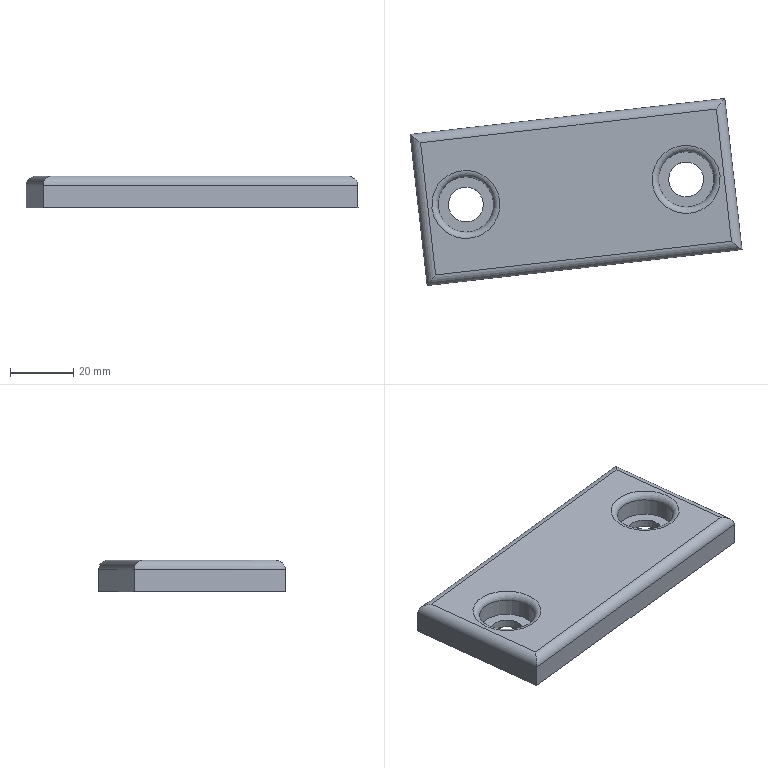Part | NX | features XQ 2 | 1 solid | 18 faces | box 104.791 x 59.012 x 10 mm | volume 43256 mm3 | plane 8 | cylinder 8 | torus 2 | commonest cylinder face diameters 6 x4 11 x2 17.5 x2
STEP:
#1=CARTESIAN_POINT('',(2747.315,315.593,-122.5));
#2=VERTEX_POINT('',#1);
#3=CARTESIAN_POINT('',(2747.315,315.593,-115.5));
#4=VERTEX_POINT('',#3);
#5=CARTESIAN_POINT('',(2747.315,315.593,-117.5));
#6=DIRECTION('',(-0.000000001,0.,1.));
#7=VECTOR('',#6,1000.);
#8=LINE('',#5,#7);
#9=EDGE_CURVE('',#2,#4,#8,.T.);
#10=ORIENTED_EDGE('',*,*,#9,.F.);
#11=CARTESIAN_POINT('',(2647.958,304.273,-122.5));
#12=VERTEX_POINT('',#11);
#13=CARTESIAN_POINT('',(2647.958,304.273,-122.5));
#14=DIRECTION('',(0.9936,0.1132,0.000000001));
#15=VECTOR('',#14,1000.);
#16=LINE('',#13,#15);
#17=EDGE_CURVE('',#12,#2,#16,.T.);
#18=ORIENTED_EDGE('',*,*,#17,.F.);
#19=CARTESIAN_POINT('',(2647.958,304.273,-115.5));
#20=VERTEX_POINT('',#19);
#21=CARTESIAN_POINT('',(2647.958,304.273,-117.5));
#22=DIRECTION('',(0.000000001,0.,-1.));
#23=VECTOR('',#22,1000.);
#24=LINE('',#21,#23);
#25=EDGE_CURVE('',#20,#12,#24,.T.);
#26=ORIENTED_EDGE('',*,*,#25,.F.);
#27=CARTESIAN_POINT('',(2647.958,304.273,-115.5));
#28=DIRECTION('',(-0.9936,-0.1132,-0.000000001));
#29=VECTOR('',#28,1000.);
#30=LINE('',#27,#29);
#31=EDGE_CURVE('',#4,#20,#30,.T.);
#32=ORIENTED_EDGE('',*,*,#31,.F.);
#33=EDGE_LOOP('',(#10,#18,#26,#32));
#34=FACE_BOUND('',#33,.T.);
#35=CARTESIAN_POINT('',(2647.958,304.273,-117.5));
#36=DIRECTION('',(-0.1132,0.9936,0.));
#37=DIRECTION('',(0.9936,0.1132,0.000000001));
#38=AXIS2_PLACEMENT_3D('',#35,#36,#37);
#39=PLANE('',#38);
#40=ADVANCED_FACE('',(#34),#39,.T.);
#41=CARTESIAN_POINT('',(2752.749,267.902,-115.5));
#42=VERTEX_POINT('',#41);
#43=CARTESIAN_POINT('',(2752.749,267.902,-122.5));
#44=VERTEX_POINT('',#43);
#45=CARTESIAN_POINT('',(2752.749,267.902,-117.5));
#46=DIRECTION('',(0.000000001,0.,-1.));
#47=VECTOR('',#46,1000.);
#48=LINE('',#45,#47);
#49=EDGE_CURVE('',#42,#44,#48,.T.);
#50=ORIENTED_EDGE('',*,*,#49,.T.);
#51=CARTESIAN_POINT('',(2750.032,291.748,-122.5));
#52=DIRECTION('',(0.1132,-0.9936,0.));
#53=VECTOR('',#52,1000.);
#54=LINE('',#51,#53);
#55=EDGE_CURVE('',#2,#44,#54,.T.);
#56=ORIENTED_EDGE('',*,*,#55,.F.);
#57=ORIENTED_EDGE('',*,*,#9,.T.);
#58=CARTESIAN_POINT('',(2750.032,291.748,-115.5));
#59=DIRECTION('',(-0.1132,0.9936,0.));
#60=VECTOR('',#59,1000.);
#61=LINE('',#58,#60);
#62=EDGE_CURVE('',#42,#4,#61,.T.);
#63=ORIENTED_EDGE('',*,*,#62,.F.);
#64=EDGE_LOOP('',(#50,#56,#57,#63));
#65=FACE_BOUND('',#64,.T.);
#66=CARTESIAN_POINT('',(2750.032,291.748,-117.5));
#67=DIRECTION('',(0.9936,0.1132,0.000000001));
#68=DIRECTION('',(0.1132,-0.9936,0.));
#69=AXIS2_PLACEMENT_3D('',#66,#67,#68);
#70=PLANE('',#69);
#71=ADVANCED_FACE('',(#65),#70,.T.);
#72=CARTESIAN_POINT('',(2724.448,288.833,-112.5));
#73=VERTEX_POINT('',#72);
#74=CARTESIAN_POINT('',(2735.129,290.05,-112.5));
#75=DIRECTION('',(-0.000000001,0.,1.));
#76=DIRECTION('',(-0.9936,-0.1132,-0.000000001));
#77=AXIS2_PLACEMENT_3D('',#74,#75,#76);
#78=CIRCLE('',#77,10.75);
#79=EDGE_CURVE('',#73,#73,#78,.T.);
#80=ORIENTED_EDGE('',*,*,#79,.F.);
#81=EDGE_LOOP('',(#80));
#82=FACE_BOUND('',#81,.T.);
#83=CARTESIAN_POINT('',(2654.898,280.908,-112.5));
#84=VERTEX_POINT('',#83);
#85=CARTESIAN_POINT('',(2665.579,282.125,-112.5));
#86=DIRECTION('',(-0.000000001,0.,1.));
#87=DIRECTION('',(-0.9936,-0.1132,-0.000000001));
#88=AXIS2_PLACEMENT_3D('',#85,#86,#87);
#89=CIRCLE('',#88,10.75);
#90=EDGE_CURVE('',#84,#84,#89,.T.);
#91=ORIENTED_EDGE('',*,*,#90,.F.);
#92=EDGE_LOOP('',(#91));
#93=FACE_BOUND('',#92,.T.);
#94=CARTESIAN_POINT('',(2749.429,270.543,-112.5));
#95=VERTEX_POINT('',#94);
#96=CARTESIAN_POINT('',(2656.033,259.902,-112.5));
#97=VERTEX_POINT('',#96);
#98=CARTESIAN_POINT('',(2653.052,259.562,-112.5));
#99=DIRECTION('',(-0.9936,-0.1132,-0.000000001));
#100=VECTOR('',#99,1000.);
#101=LINE('',#98,#100);
#102=EDGE_CURVE('',#95,#97,#101,.T.);
#103=ORIENTED_EDGE('',*,*,#102,.F.);
#104=CARTESIAN_POINT('',(2744.674,312.273,-112.5));
#105=VERTEX_POINT('',#104);
#106=CARTESIAN_POINT('',(2747.052,291.408,-112.5));
#107=DIRECTION('',(0.1132,-0.9936,0.));
#108=VECTOR('',#107,1000.);
#109=LINE('',#106,#108);
#110=EDGE_CURVE('',#105,#95,#109,.T.);
#111=ORIENTED_EDGE('',*,*,#110,.F.);
#112=CARTESIAN_POINT('',(2651.279,301.632,-112.5));
#113=VERTEX_POINT('',#112);
#114=CARTESIAN_POINT('',(2648.298,301.292,-112.5));
#115=DIRECTION('',(0.9936,0.1132,0.000000001));
#116=VECTOR('',#115,1000.);
#117=LINE('',#114,#116);
#118=EDGE_CURVE('',#113,#105,#117,.T.);
#119=ORIENTED_EDGE('',*,*,#118,.F.);
#120=CARTESIAN_POINT('',(2653.656,280.767,-112.5));
#121=DIRECTION('',(-0.1132,0.9936,0.));
#122=VECTOR('',#121,1000.);
#123=LINE('',#120,#122);
#124=EDGE_CURVE('',#97,#113,#123,.T.);
#125=ORIENTED_EDGE('',*,*,#124,.F.);
#126=EDGE_LOOP('',(#103,#111,#119,#125));
#127=FACE_BOUND('',#126,.T.);
#128=CARTESIAN_POINT('',(2650.675,280.427,-112.5));
#129=DIRECTION('',(-0.000000001,0.,1.));
#130=DIRECTION('',(0.9936,0.1132,0.000000001));
#131=AXIS2_PLACEMENT_3D('',#128,#129,#130);
#132=PLANE('',#131);
#133=ADVANCED_FACE('',(#82,#93,#127),#132,.T.);
#134=CARTESIAN_POINT('',(2653.392,256.582,-122.5));
#135=VERTEX_POINT('',#134);
#136=CARTESIAN_POINT('',(2653.392,256.582,-115.5));
#137=VERTEX_POINT('',#136);
#138=CARTESIAN_POINT('',(2653.392,256.582,-117.5));
#139=DIRECTION('',(-0.000000001,0.,1.));
#140=VECTOR('',#139,1000.);
#141=LINE('',#138,#140);
#142=EDGE_CURVE('',#135,#137,#141,.T.);
#143=ORIENTED_EDGE('',*,*,#142,.F.);
#144=CARTESIAN_POINT('',(2653.392,256.582,-122.5));
#145=DIRECTION('',(0.9936,0.1132,0.000000001));
#146=VECTOR('',#145,1000.);
#147=LINE('',#144,#146);
#148=EDGE_CURVE('',#135,#44,#147,.T.);
#149=ORIENTED_EDGE('',*,*,#148,.T.);
#150=ORIENTED_EDGE('',*,*,#49,.F.);
#151=CARTESIAN_POINT('',(2653.392,256.582,-115.5));
#152=DIRECTION('',(0.9936,0.1132,0.000000001));
#153=VECTOR('',#152,1000.);
#154=LINE('',#151,#153);
#155=EDGE_CURVE('',#137,#42,#154,.T.);
#156=ORIENTED_EDGE('',*,*,#155,.F.);
#157=EDGE_LOOP('',(#143,#149,#150,#156));
#158=FACE_BOUND('',#157,.T.);
#159=CARTESIAN_POINT('',(2653.392,256.582,-117.5));
#160=DIRECTION('',(0.1132,-0.9936,0.));
#161=DIRECTION('',(-0.9936,-0.1132,-0.000000001));
#162=AXIS2_PLACEMENT_3D('',#159,#160,#161);
#163=PLANE('',#162);
#164=ADVANCED_FACE('',(#158),#163,.T.);
#165=CARTESIAN_POINT('',(2729.664,289.427,-122.5));
#166=VERTEX_POINT('',#165);
#167=CARTESIAN_POINT('',(2735.129,290.05,-122.5));
#168=DIRECTION('',(0.000000001,0.,-1.));
#169=DIRECTION('',(-0.9936,-0.1132,-0.000000001));
#170=AXIS2_PLACEMENT_3D('',#167,#168,#169);
#171=CIRCLE('',#170,5.5);
#172=EDGE_CURVE('',#166,#166,#171,.T.);
#173=ORIENTED_EDGE('',*,*,#172,.F.);
#174=EDGE_LOOP('',(#173));
#175=FACE_BOUND('',#174,.T.);
#176=CARTESIAN_POINT('',(2660.114,281.503,-122.5));
#177=VERTEX_POINT('',#176);
#178=CARTESIAN_POINT('',(2665.579,282.125,-122.5));
#179=DIRECTION('',(0.000000001,0.,-1.));
#180=DIRECTION('',(-0.9936,-0.1132,-0.000000001));
#181=AXIS2_PLACEMENT_3D('',#178,#179,#180);
#182=CIRCLE('',#181,5.5);
#183=EDGE_CURVE('',#177,#177,#182,.T.);
#184=ORIENTED_EDGE('',*,*,#183,.F.);
#185=EDGE_LOOP('',(#184));
#186=FACE_BOUND('',#185,.T.);
#187=ORIENTED_EDGE('',*,*,#148,.F.);
#188=CARTESIAN_POINT('',(2650.675,280.427,-122.5));
#189=DIRECTION('',(-0.1132,0.9936,0.));
#190=VECTOR('',#189,1000.);
#191=LINE('',#188,#190);
#192=EDGE_CURVE('',#135,#12,#191,.T.);
#193=ORIENTED_EDGE('',*,*,#192,.T.);
#194=ORIENTED_EDGE('',*,*,#17,.T.);
#195=ORIENTED_EDGE('',*,*,#55,.T.);
#196=EDGE_LOOP('',(#187,#193,#194,#195));
#197=FACE_BOUND('',#196,.T.);
#198=CARTESIAN_POINT('',(2650.675,280.427,-122.5));
#199=DIRECTION('',(0.000000001,0.,-1.));
#200=DIRECTION('',(-0.9936,-0.1132,-0.000000001));
#201=AXIS2_PLACEMENT_3D('',#198,#199,#200);
#202=PLANE('',#201);
#203=ADVANCED_FACE('',(#175,#186,#197),#202,.T.);
#204=ORIENTED_EDGE('',*,*,#25,.T.);
#205=ORIENTED_EDGE('',*,*,#192,.F.);
#206=ORIENTED_EDGE('',*,*,#142,.T.);
#207=CARTESIAN_POINT('',(2650.675,280.427,-115.5));
#208=DIRECTION('',(0.1132,-0.9936,0.));
#209=VECTOR('',#208,1000.);
#210=LINE('',#207,#209);
#211=EDGE_CURVE('',#20,#137,#210,.T.);
#212=ORIENTED_EDGE('',*,*,#211,.F.);
#213=EDGE_LOOP('',(#204,#205,#206,#212));
#214=FACE_BOUND('',#213,.T.);
#215=CARTESIAN_POINT('',(2650.675,280.427,-117.5));
#216=DIRECTION('',(-0.9936,-0.1132,-0.000000001));
#217=DIRECTION('',(-0.1132,0.9936,0.));
#218=AXIS2_PLACEMENT_3D('',#215,#216,#217);
#219=PLANE('',#218);
#220=ADVANCED_FACE('',(#214),#219,.T.);
#221=CARTESIAN_POINT('',(2744.674,312.273,-115.5));
#222=DIRECTION('',(0.7826,-0.6225,0.000000001));
#223=DIRECTION('',(0.6225,0.7826,0.));
#224=AXIS2_PLACEMENT_3D('',#221,#222,#223);
#225=ELLIPSE('',#224,4.243,3.);
#226=EDGE_CURVE('',#4,#105,#225,.T.);
#227=ORIENTED_EDGE('',*,*,#226,.T.);
#228=ORIENTED_EDGE('',*,*,#110,.T.);
#229=CARTESIAN_POINT('',(2749.429,270.543,-115.5));
#230=DIRECTION('',(0.6225,0.7826,0.));
#231=DIRECTION('',(0.7826,-0.6225,0.000000001));
#232=AXIS2_PLACEMENT_3D('',#229,#230,#231);
#233=ELLIPSE('',#232,4.243,3.);
#234=EDGE_CURVE('',#95,#42,#233,.T.);
#235=ORIENTED_EDGE('',*,*,#234,.T.);
#236=ORIENTED_EDGE('',*,*,#62,.T.);
#237=EDGE_LOOP('',(#227,#228,#235,#236));
#238=FACE_BOUND('',#237,.T.);
#239=CARTESIAN_POINT('',(2747.052,291.408,-115.5));
#240=DIRECTION('',(0.1132,-0.9936,0.));
#241=DIRECTION('',(-0.9936,-0.1132,-0.000000001));
#242=AXIS2_PLACEMENT_3D('',#239,#240,#241);
#243=CYLINDRICAL_SURFACE('',#242,3.);
#244=ADVANCED_FACE('',(#238),#243,.T.);
#245=ORIENTED_EDGE('',*,*,#234,.F.);
#246=ORIENTED_EDGE('',*,*,#102,.T.);
#247=CARTESIAN_POINT('',(2656.033,259.902,-115.5));
#248=DIRECTION('',(0.7826,-0.6225,0.000000001));
#249=DIRECTION('',(0.6225,0.7826,0.));
#250=AXIS2_PLACEMENT_3D('',#247,#248,#249);
#251=ELLIPSE('',#250,4.243,3.);
#252=EDGE_CURVE('',#97,#137,#251,.T.);
#253=ORIENTED_EDGE('',*,*,#252,.T.);
#254=ORIENTED_EDGE('',*,*,#155,.T.);
#255=EDGE_LOOP('',(#245,#246,#253,#254));
#256=FACE_BOUND('',#255,.T.);
#257=CARTESIAN_POINT('',(2653.052,259.562,-115.5));
#258=DIRECTION('',(0.9936,0.1132,0.000000001));
#259=DIRECTION('',(0.1132,-0.9936,0.));
#260=AXIS2_PLACEMENT_3D('',#257,#258,#259);
#261=CYLINDRICAL_SURFACE('',#260,3.);
#262=ADVANCED_FACE('',(#256),#261,.T.);
#263=ORIENTED_EDGE('',*,*,#226,.F.);
#264=ORIENTED_EDGE('',*,*,#31,.T.);
#265=CARTESIAN_POINT('',(2651.279,301.632,-115.5));
#266=DIRECTION('',(0.6225,0.7826,0.));
#267=DIRECTION('',(-0.7826,0.6225,-0.000000001));
#268=AXIS2_PLACEMENT_3D('',#265,#266,#267);
#269=ELLIPSE('',#268,4.243,3.);
#270=EDGE_CURVE('',#20,#113,#269,.T.);
#271=ORIENTED_EDGE('',*,*,#270,.T.);
#272=ORIENTED_EDGE('',*,*,#118,.T.);
#273=EDGE_LOOP('',(#263,#264,#271,#272));
#274=FACE_BOUND('',#273,.T.);
#275=CARTESIAN_POINT('',(2648.298,301.292,-115.5));
#276=DIRECTION('',(0.9936,0.1132,0.000000001));
#277=DIRECTION('',(0.1132,-0.9936,0.));
#278=AXIS2_PLACEMENT_3D('',#275,#276,#277);
#279=CYLINDRICAL_SURFACE('',#278,3.);
#280=ADVANCED_FACE('',(#274),#279,.T.);
#281=ORIENTED_EDGE('',*,*,#252,.F.);
#282=ORIENTED_EDGE('',*,*,#124,.T.);
#283=ORIENTED_EDGE('',*,*,#270,.F.);
#284=ORIENTED_EDGE('',*,*,#211,.T.);
#285=EDGE_LOOP('',(#281,#282,#283,#284));
#286=FACE_BOUND('',#285,.T.);
#287=CARTESIAN_POINT('',(2653.656,280.767,-115.5));
#288=DIRECTION('',(-0.1132,0.9936,0.));
#289=DIRECTION('',(0.9936,0.1132,0.000000001));
#290=AXIS2_PLACEMENT_3D('',#287,#288,#289);
#291=CYLINDRICAL_SURFACE('',#290,3.);
#292=ADVANCED_FACE('',(#286),#291,.T.);
#293=CARTESIAN_POINT('',(2671.043,282.748,-120.));
#294=VERTEX_POINT('',#293);
#295=CARTESIAN_POINT('',(2665.579,282.125,-120.));
#296=DIRECTION('',(-0.000000001,0.,1.));
#297=DIRECTION('',(0.9936,0.1132,0.000000001));
#298=AXIS2_PLACEMENT_3D('',#295,#296,#297);
#299=CIRCLE('',#298,5.5);
#300=EDGE_CURVE('',#294,#294,#299,.T.);
#301=ORIENTED_EDGE('',*,*,#300,.F.);
#302=EDGE_LOOP('',(#301));
#303=FACE_BOUND('',#302,.T.);
#304=CARTESIAN_POINT('',(2656.885,281.135,-120.));
#305=VERTEX_POINT('',#304);
#306=CARTESIAN_POINT('',(2665.579,282.125,-120.));
#307=DIRECTION('',(-0.000000001,0.,1.));
#308=DIRECTION('',(-0.9936,-0.1132,-0.000000001));
#309=AXIS2_PLACEMENT_3D('',#306,#307,#308);
#310=CIRCLE('',#309,8.75);
#311=EDGE_CURVE('',#305,#305,#310,.T.);
#312=ORIENTED_EDGE('',*,*,#311,.T.);
#313=EDGE_LOOP('',(#312));
#314=FACE_BOUND('',#313,.T.);
#315=CARTESIAN_POINT('',(2665.579,282.125,-120.));
#316=DIRECTION('',(0.000000001,0.,-1.));
#317=DIRECTION('',(-0.9936,-0.1132,-0.000000001));
#318=AXIS2_PLACEMENT_3D('',#315,#316,#317);
#319=PLANE('',#318);
#320=ADVANCED_FACE('',(#303,#314),#319,.F.);
#321=CARTESIAN_POINT('',(2656.885,281.135,-114.5));
#322=VERTEX_POINT('',#321);
#323=CARTESIAN_POINT('',(2665.579,282.125,-114.5));
#324=DIRECTION('',(0.000000001,0.,-1.));
#325=DIRECTION('',(-0.9936,-0.1132,-0.000000001));
#326=AXIS2_PLACEMENT_3D('',#323,#324,#325);
#327=CIRCLE('',#326,8.75);
#328=EDGE_CURVE('',#322,#322,#327,.T.);
#329=ORIENTED_EDGE('',*,*,#328,.F.);
#330=EDGE_LOOP('',(#329));
#331=FACE_BOUND('',#330,.T.);
#332=ORIENTED_EDGE('',*,*,#311,.F.);
#333=EDGE_LOOP('',(#332));
#334=FACE_BOUND('',#333,.T.);
#335=CARTESIAN_POINT('',(2665.579,282.125,-112.5));
#336=DIRECTION('',(0.000000001,0.,-1.));
#337=DIRECTION('',(-0.9936,-0.1132,-0.000000001));
#338=AXIS2_PLACEMENT_3D('',#335,#336,#337);
#339=CYLINDRICAL_SURFACE('',#338,8.75);
#340=ADVANCED_FACE('',(#331,#334),#339,.F.);
#341=ORIENTED_EDGE('',*,*,#183,.T.);
#342=EDGE_LOOP('',(#341));
#343=FACE_BOUND('',#342,.T.);
#344=ORIENTED_EDGE('',*,*,#300,.T.);
#345=EDGE_LOOP('',(#344));
#346=FACE_BOUND('',#345,.T.);
#347=CARTESIAN_POINT('',(2665.579,282.125,-112.5));
#348=DIRECTION('',(0.000000001,0.,-1.));
#349=DIRECTION('',(-0.9936,-0.1132,-0.000000001));
#350=AXIS2_PLACEMENT_3D('',#347,#348,#349);
#351=CYLINDRICAL_SURFACE('',#350,5.5);
#352=ADVANCED_FACE('',(#343,#346),#351,.F.);
#353=CARTESIAN_POINT('',(2740.593,290.672,-120.));
#354=VERTEX_POINT('',#353);
#355=CARTESIAN_POINT('',(2735.129,290.05,-120.));
#356=DIRECTION('',(-0.000000001,0.,1.));
#357=DIRECTION('',(0.9936,0.1132,0.000000001));
#358=AXIS2_PLACEMENT_3D('',#355,#356,#357);
#359=CIRCLE('',#358,5.5);
#360=EDGE_CURVE('',#354,#354,#359,.T.);
#361=ORIENTED_EDGE('',*,*,#360,.F.);
#362=EDGE_LOOP('',(#361));
#363=FACE_BOUND('',#362,.T.);
#364=CARTESIAN_POINT('',(2726.435,289.059,-120.));
#365=VERTEX_POINT('',#364);
#366=CARTESIAN_POINT('',(2735.129,290.05,-120.));
#367=DIRECTION('',(-0.000000001,0.,1.));
#368=DIRECTION('',(-0.9936,-0.1132,-0.000000001));
#369=AXIS2_PLACEMENT_3D('',#366,#367,#368);
#370=CIRCLE('',#369,8.75);
#371=EDGE_CURVE('',#365,#365,#370,.T.);
#372=ORIENTED_EDGE('',*,*,#371,.T.);
#373=EDGE_LOOP('',(#372));
#374=FACE_BOUND('',#373,.T.);
#375=CARTESIAN_POINT('',(2735.129,290.05,-120.));
#376=DIRECTION('',(0.000000001,0.,-1.));
#377=DIRECTION('',(-0.9936,-0.1132,-0.000000001));
#378=AXIS2_PLACEMENT_3D('',#375,#376,#377);
#379=PLANE('',#378);
#380=ADVANCED_FACE('',(#363,#374),#379,.F.);
#381=CARTESIAN_POINT('',(2726.435,289.059,-114.5));
#382=VERTEX_POINT('',#381);
#383=CARTESIAN_POINT('',(2735.129,290.05,-114.5));
#384=DIRECTION('',(0.000000001,0.,-1.));
#385=DIRECTION('',(-0.9936,-0.1132,-0.000000001));
#386=AXIS2_PLACEMENT_3D('',#383,#384,#385);
#387=CIRCLE('',#386,8.75);
#388=EDGE_CURVE('',#382,#382,#387,.T.);
#389=ORIENTED_EDGE('',*,*,#388,.F.);
#390=EDGE_LOOP('',(#389));
#391=FACE_BOUND('',#390,.T.);
#392=ORIENTED_EDGE('',*,*,#371,.F.);
#393=EDGE_LOOP('',(#392));
#394=FACE_BOUND('',#393,.T.);
#395=CARTESIAN_POINT('',(2735.129,290.05,-112.5));
#396=DIRECTION('',(0.000000001,0.,-1.));
#397=DIRECTION('',(-0.9936,-0.1132,-0.000000001));
#398=AXIS2_PLACEMENT_3D('',#395,#396,#397);
#399=CYLINDRICAL_SURFACE('',#398,8.75);
#400=ADVANCED_FACE('',(#391,#394),#399,.F.);
#401=ORIENTED_EDGE('',*,*,#172,.T.);
#402=EDGE_LOOP('',(#401));
#403=FACE_BOUND('',#402,.T.);
#404=ORIENTED_EDGE('',*,*,#360,.T.);
#405=EDGE_LOOP('',(#404));
#406=FACE_BOUND('',#405,.T.);
#407=CARTESIAN_POINT('',(2735.129,290.05,-112.5));
#408=DIRECTION('',(0.000000001,0.,-1.));
#409=DIRECTION('',(-0.9936,-0.1132,-0.000000001));
#410=AXIS2_PLACEMENT_3D('',#407,#408,#409);
#411=CYLINDRICAL_SURFACE('',#410,5.5);
#412=ADVANCED_FACE('',(#403,#406),#411,.F.);
#413=ORIENTED_EDGE('',*,*,#328,.T.);
#414=EDGE_LOOP('',(#413));
#415=FACE_BOUND('',#414,.T.);
#416=ORIENTED_EDGE('',*,*,#90,.T.);
#417=EDGE_LOOP('',(#416));
#418=FACE_BOUND('',#417,.T.);
#419=CARTESIAN_POINT('',(2665.579,282.125,-114.5));
#420=DIRECTION('',(-0.000000001,0.,1.));
#421=DIRECTION('',(0.9936,0.1132,0.000000001));
#422=AXIS2_PLACEMENT_3D('',#419,#420,#421);
#423=TOROIDAL_SURFACE('',#422,10.75,2.);
#424=ADVANCED_FACE('',(#415,#418),#423,.T.);
#425=ORIENTED_EDGE('',*,*,#388,.T.);
#426=EDGE_LOOP('',(#425));
#427=FACE_BOUND('',#426,.T.);
#428=ORIENTED_EDGE('',*,*,#79,.T.);
#429=EDGE_LOOP('',(#428));
#430=FACE_BOUND('',#429,.T.);
#431=CARTESIAN_POINT('',(2735.129,290.05,-114.5));
#432=DIRECTION('',(-0.000000001,0.,1.));
#433=DIRECTION('',(0.9936,0.1132,0.000000001));
#434=AXIS2_PLACEMENT_3D('',#431,#432,#433);
#435=TOROIDAL_SURFACE('',#434,10.75,2.);
#436=ADVANCED_FACE('',(#427,#430),#435,.T.);
#437=CLOSED_SHELL('',(#40,#71,#133,#164,#203,#220,#244,#262,#280,#292,#320,#340,#352,#380,#400,#412,#424,#436));
#438=MANIFOLD_SOLID_BREP('',#437);
#439=(LENGTH_UNIT()NAMED_UNIT(*)SI_UNIT(.MILLI.,.METRE.));
#440=UNCERTAINTY_MEASURE_WITH_UNIT(LENGTH_MEASURE(0.00001),#439,'','');
#441=(NAMED_UNIT(*)PLANE_ANGLE_UNIT()SI_UNIT($,.RADIAN.));
#442=(NAMED_UNIT(*)SI_UNIT($,.STERADIAN.)SOLID_ANGLE_UNIT());
#443=(GEOMETRIC_REPRESENTATION_CONTEXT(3)GLOBAL_UNCERTAINTY_ASSIGNED_CONTEXT((#440))GLOBAL_UNIT_ASSIGNED_CONTEXT((#439,#441,#442))REPRESENTATION_CONTEXT('',''));
#444=ADVANCED_BREP_SHAPE_REPRESENTATION('',(#438),#443);